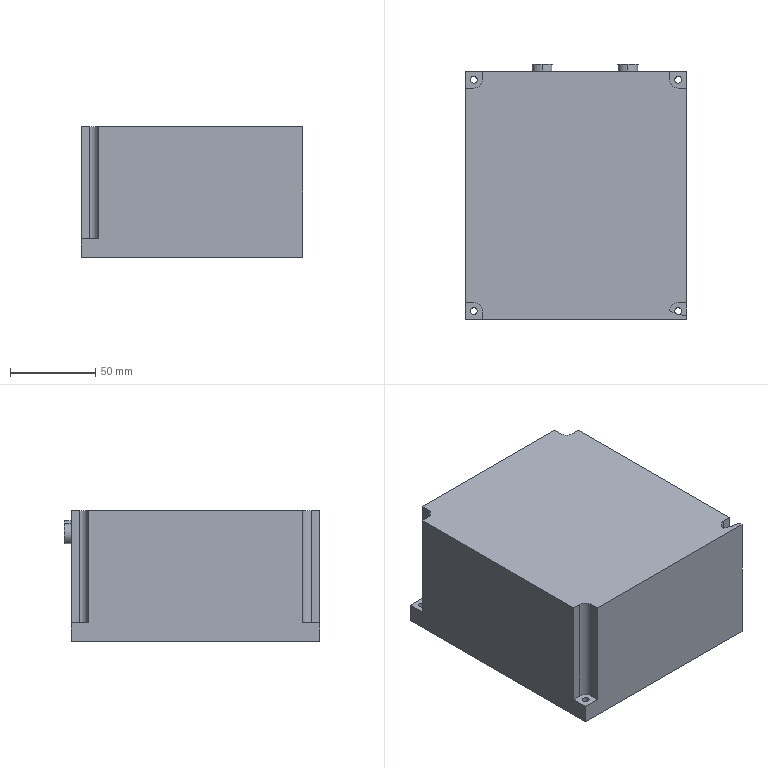Part | SolidWorks | features ICE 2, Extrusion 1 | 1 solid | 37 faces | box 130 x 150 x 77 mm | volume 1439024 mm3 | plane 21 | cylinder 16 | commonest cylinder face diameters 4 x8 10 x4 11.874 x2 11.972 x2
STEP:
#1=CARTESIAN_POINT('',(95.565,150.,59.228));
#2=VERTEX_POINT('',#1);
#3=CARTESIAN_POINT('',(95.565,150.,71.102));
#4=VERTEX_POINT('',#3);
#5=CARTESIAN_POINT('',(95.565,150.,65.165));
#6=DIRECTION('',(0.,-1.,0.));
#7=DIRECTION('',(0.,0.,-1.));
#8=AXIS2_PLACEMENT_3D('',#5,#6,#7);
#9=CIRCLE('',#8,5.937);
#10=EDGE_CURVE('',#2,#4,#9,.T.);
#11=ORIENTED_EDGE('',*,*,#10,.T.);
#12=CARTESIAN_POINT('',(95.565,146.,71.102));
#13=VERTEX_POINT('',#12);
#14=CARTESIAN_POINT('',(95.565,150.,71.102));
#15=DIRECTION('',(0.,-1.,0.));
#16=VECTOR('',#15,1000.);
#17=LINE('',#14,#16);
#18=EDGE_CURVE('',#4,#13,#17,.T.);
#19=ORIENTED_EDGE('',*,*,#18,.T.);
#20=CARTESIAN_POINT('',(95.565,146.,59.228));
#21=VERTEX_POINT('',#20);
#22=CARTESIAN_POINT('',(95.565,146.,65.165));
#23=DIRECTION('',(0.,-1.,0.));
#24=DIRECTION('',(0.,0.,-1.));
#25=AXIS2_PLACEMENT_3D('',#22,#23,#24);
#26=CIRCLE('',#25,5.937);
#27=EDGE_CURVE('',#21,#13,#26,.T.);
#28=ORIENTED_EDGE('',*,*,#27,.F.);
#29=CARTESIAN_POINT('',(95.565,150.,59.228));
#30=DIRECTION('',(0.,-1.,0.));
#31=VECTOR('',#30,1000.);
#32=LINE('',#29,#31);
#33=EDGE_CURVE('',#2,#21,#32,.T.);
#34=ORIENTED_EDGE('',*,*,#33,.F.);
#35=EDGE_LOOP('',(#11,#19,#28,#34));
#36=FACE_OUTER_BOUND('',#35,.T.);
#37=CARTESIAN_POINT('',(95.565,150.,65.165));
#38=DIRECTION('',(0.,-1.,0.));
#39=DIRECTION('',(0.,0.,-1.));
#40=AXIS2_PLACEMENT_3D('',#37,#38,#39);
#41=CYLINDRICAL_SURFACE('',#40,5.937);
#42=ADVANCED_FACE('',(#36),#41,.T.);
#43=CARTESIAN_POINT('',(45.097,150.,57.435));
#44=VERTEX_POINT('',#43);
#45=CARTESIAN_POINT('',(45.097,150.,69.406));
#46=VERTEX_POINT('',#45);
#47=CARTESIAN_POINT('',(45.097,150.,63.42));
#48=DIRECTION('',(0.,-1.,0.));
#49=DIRECTION('',(0.,0.,-1.));
#50=AXIS2_PLACEMENT_3D('',#47,#48,#49);
#51=CIRCLE('',#50,5.986);
#52=EDGE_CURVE('',#44,#46,#51,.T.);
#53=ORIENTED_EDGE('',*,*,#52,.T.);
#54=CARTESIAN_POINT('',(45.097,146.,69.406));
#55=VERTEX_POINT('',#54);
#56=CARTESIAN_POINT('',(45.097,150.,69.406));
#57=DIRECTION('',(0.,-1.,0.));
#58=VECTOR('',#57,1000.);
#59=LINE('',#56,#58);
#60=EDGE_CURVE('',#46,#55,#59,.T.);
#61=ORIENTED_EDGE('',*,*,#60,.T.);
#62=CARTESIAN_POINT('',(45.097,146.,57.435));
#63=VERTEX_POINT('',#62);
#64=CARTESIAN_POINT('',(45.097,146.,63.42));
#65=DIRECTION('',(0.,-1.,0.));
#66=DIRECTION('',(0.,0.,-1.));
#67=AXIS2_PLACEMENT_3D('',#64,#65,#66);
#68=CIRCLE('',#67,5.986);
#69=EDGE_CURVE('',#63,#55,#68,.T.);
#70=ORIENTED_EDGE('',*,*,#69,.F.);
#71=CARTESIAN_POINT('',(45.097,150.,57.435));
#72=DIRECTION('',(0.,-1.,0.));
#73=VECTOR('',#72,1000.);
#74=LINE('',#71,#73);
#75=EDGE_CURVE('',#44,#63,#74,.T.);
#76=ORIENTED_EDGE('',*,*,#75,.F.);
#77=EDGE_LOOP('',(#53,#61,#70,#76));
#78=FACE_OUTER_BOUND('',#77,.T.);
#79=CARTESIAN_POINT('',(45.097,150.,63.42));
#80=DIRECTION('',(0.,-1.,0.));
#81=DIRECTION('',(0.,0.,-1.));
#82=AXIS2_PLACEMENT_3D('',#79,#80,#81);
#83=CYLINDRICAL_SURFACE('',#82,5.986);
#84=ADVANCED_FACE('',(#78),#83,.T.);
#85=CARTESIAN_POINT('',(125.827,3.179,11.));
#86=VERTEX_POINT('',#85);
#87=CARTESIAN_POINT('',(127.,5.,11.));
#88=VERTEX_POINT('',#87);
#89=CARTESIAN_POINT('',(125.,5.,11.));
#90=DIRECTION('',(0.,0.,1.));
#91=DIRECTION('',(1.,0.,0.));
#92=AXIS2_PLACEMENT_3D('',#89,#90,#91);
#93=CIRCLE('',#92,2.);
#94=EDGE_CURVE('',#86,#88,#93,.T.);
#95=ORIENTED_EDGE('',*,*,#94,.T.);
#96=CARTESIAN_POINT('',(127.,5.,0.));
#97=VERTEX_POINT('',#96);
#98=CARTESIAN_POINT('',(127.,5.,77.));
#99=DIRECTION('',(0.,0.,-1.));
#100=VECTOR('',#99,1000.);
#101=LINE('',#98,#100);
#102=EDGE_CURVE('',#88,#97,#101,.T.);
#103=ORIENTED_EDGE('',*,*,#102,.T.);
#104=CARTESIAN_POINT('',(123.,5.,0.));
#105=VERTEX_POINT('',#104);
#106=CARTESIAN_POINT('',(125.,5.,0.));
#107=DIRECTION('',(0.,0.,1.));
#108=DIRECTION('',(1.,0.,0.));
#109=AXIS2_PLACEMENT_3D('',#106,#107,#108);
#110=CIRCLE('',#109,2.);
#111=EDGE_CURVE('',#105,#97,#110,.T.);
#112=ORIENTED_EDGE('',*,*,#111,.F.);
#113=CARTESIAN_POINT('',(123.,5.,11.));
#114=VERTEX_POINT('',#113);
#115=CARTESIAN_POINT('',(123.,5.,77.));
#116=DIRECTION('',(0.,0.,-1.));
#117=VECTOR('',#116,1000.);
#118=LINE('',#115,#117);
#119=EDGE_CURVE('',#114,#105,#118,.T.);
#120=ORIENTED_EDGE('',*,*,#119,.F.);
#121=CARTESIAN_POINT('',(123.283,3.974,11.));
#122=VERTEX_POINT('',#121);
#123=CARTESIAN_POINT('',(125.,5.,11.));
#124=DIRECTION('',(0.,0.,1.));
#125=DIRECTION('',(1.,0.,0.));
#126=AXIS2_PLACEMENT_3D('',#123,#124,#125);
#127=CIRCLE('',#126,2.);
#128=EDGE_CURVE('',#114,#122,#127,.T.);
#129=ORIENTED_EDGE('',*,*,#128,.T.);
#130=CARTESIAN_POINT('',(123.283,3.974,77.));
#131=VERTEX_POINT('',#130);
#132=CARTESIAN_POINT('',(123.283,3.974,77.));
#133=DIRECTION('',(0.,0.,-1.));
#134=VECTOR('',#133,1000.);
#135=LINE('',#132,#134);
#136=EDGE_CURVE('',#131,#122,#135,.T.);
#137=ORIENTED_EDGE('',*,*,#136,.F.);
#138=CARTESIAN_POINT('',(125.827,3.179,77.));
#139=VERTEX_POINT('',#138);
#140=CARTESIAN_POINT('',(125.,5.,77.));
#141=DIRECTION('',(0.,0.,1.));
#142=DIRECTION('',(1.,0.,0.));
#143=AXIS2_PLACEMENT_3D('',#140,#141,#142);
#144=CIRCLE('',#143,2.);
#145=EDGE_CURVE('',#131,#139,#144,.T.);
#146=ORIENTED_EDGE('',*,*,#145,.T.);
#147=CARTESIAN_POINT('',(125.827,3.179,77.));
#148=DIRECTION('',(0.,0.,1.));
#149=VECTOR('',#148,1000.);
#150=LINE('',#147,#149);
#151=EDGE_CURVE('',#86,#139,#150,.T.);
#152=ORIENTED_EDGE('',*,*,#151,.F.);
#153=EDGE_LOOP('',(#95,#103,#112,#120,#129,#137,#146,#152));
#154=FACE_OUTER_BOUND('',#153,.T.);
#155=CARTESIAN_POINT('',(125.,5.,77.));
#156=DIRECTION('',(0.,0.,-1.));
#157=DIRECTION('',(-1.,0.,0.));
#158=AXIS2_PLACEMENT_3D('',#155,#156,#157);
#159=CYLINDRICAL_SURFACE('',#158,2.);
#160=ADVANCED_FACE('',(#154),#159,.F.);
#161=CARTESIAN_POINT('',(123.,141.,11.));
#162=VERTEX_POINT('',#161);
#163=CARTESIAN_POINT('',(127.,141.,11.));
#164=VERTEX_POINT('',#163);
#165=CARTESIAN_POINT('',(125.,141.,11.));
#166=DIRECTION('',(0.,0.,1.));
#167=DIRECTION('',(1.,0.,0.));
#168=AXIS2_PLACEMENT_3D('',#165,#166,#167);
#169=CIRCLE('',#168,2.);
#170=EDGE_CURVE('',#162,#164,#169,.T.);
#171=ORIENTED_EDGE('',*,*,#170,.T.);
#172=CARTESIAN_POINT('',(127.,141.,0.));
#173=VERTEX_POINT('',#172);
#174=CARTESIAN_POINT('',(127.,141.,77.));
#175=DIRECTION('',(0.,0.,-1.));
#176=VECTOR('',#175,1000.);
#177=LINE('',#174,#176);
#178=EDGE_CURVE('',#164,#173,#177,.T.);
#179=ORIENTED_EDGE('',*,*,#178,.T.);
#180=CARTESIAN_POINT('',(123.,141.,0.));
#181=VERTEX_POINT('',#180);
#182=CARTESIAN_POINT('',(125.,141.,0.));
#183=DIRECTION('',(0.,0.,1.));
#184=DIRECTION('',(1.,0.,0.));
#185=AXIS2_PLACEMENT_3D('',#182,#183,#184);
#186=CIRCLE('',#185,2.);
#187=EDGE_CURVE('',#181,#173,#186,.T.);
#188=ORIENTED_EDGE('',*,*,#187,.F.);
#189=CARTESIAN_POINT('',(123.,141.,77.));
#190=DIRECTION('',(0.,0.,-1.));
#191=VECTOR('',#190,1000.);
#192=LINE('',#189,#191);
#193=EDGE_CURVE('',#162,#181,#192,.T.);
#194=ORIENTED_EDGE('',*,*,#193,.F.);
#195=EDGE_LOOP('',(#171,#179,#188,#194));
#196=FACE_OUTER_BOUND('',#195,.T.);
#197=CARTESIAN_POINT('',(125.,141.,77.));
#198=DIRECTION('',(0.,0.,-1.));
#199=DIRECTION('',(-1.,0.,0.));
#200=AXIS2_PLACEMENT_3D('',#197,#198,#199);
#201=CYLINDRICAL_SURFACE('',#200,2.);
#202=ADVANCED_FACE('',(#196),#201,.F.);
#203=CARTESIAN_POINT('',(3.,5.,11.));
#204=VERTEX_POINT('',#203);
#205=CARTESIAN_POINT('',(7.,5.,11.));
#206=VERTEX_POINT('',#205);
#207=CARTESIAN_POINT('',(5.,5.,11.));
#208=DIRECTION('',(0.,0.,1.));
#209=DIRECTION('',(1.,0.,0.));
#210=AXIS2_PLACEMENT_3D('',#207,#208,#209);
#211=CIRCLE('',#210,2.);
#212=EDGE_CURVE('',#204,#206,#211,.T.);
#213=ORIENTED_EDGE('',*,*,#212,.T.);
#214=CARTESIAN_POINT('',(7.,5.,0.));
#215=VERTEX_POINT('',#214);
#216=CARTESIAN_POINT('',(7.,5.,77.));
#217=DIRECTION('',(0.,0.,-1.));
#218=VECTOR('',#217,1000.);
#219=LINE('',#216,#218);
#220=EDGE_CURVE('',#206,#215,#219,.T.);
#221=ORIENTED_EDGE('',*,*,#220,.T.);
#222=CARTESIAN_POINT('',(3.,5.,0.));
#223=VERTEX_POINT('',#222);
#224=CARTESIAN_POINT('',(5.,5.,0.));
#225=DIRECTION('',(0.,0.,1.));
#226=DIRECTION('',(1.,0.,0.));
#227=AXIS2_PLACEMENT_3D('',#224,#225,#226);
#228=CIRCLE('',#227,2.);
#229=EDGE_CURVE('',#223,#215,#228,.T.);
#230=ORIENTED_EDGE('',*,*,#229,.F.);
#231=CARTESIAN_POINT('',(3.,5.,77.));
#232=DIRECTION('',(0.,0.,-1.));
#233=VECTOR('',#232,1000.);
#234=LINE('',#231,#233);
#235=EDGE_CURVE('',#204,#223,#234,.T.);
#236=ORIENTED_EDGE('',*,*,#235,.F.);
#237=EDGE_LOOP('',(#213,#221,#230,#236));
#238=FACE_OUTER_BOUND('',#237,.T.);
#239=CARTESIAN_POINT('',(5.,5.,77.));
#240=DIRECTION('',(0.,0.,-1.));
#241=DIRECTION('',(-1.,0.,0.));
#242=AXIS2_PLACEMENT_3D('',#239,#240,#241);
#243=CYLINDRICAL_SURFACE('',#242,2.);
#244=ADVANCED_FACE('',(#238),#243,.F.);
#245=CARTESIAN_POINT('',(3.,141.,11.));
#246=VERTEX_POINT('',#245);
#247=CARTESIAN_POINT('',(7.,141.,11.));
#248=VERTEX_POINT('',#247);
#249=CARTESIAN_POINT('',(5.,141.,11.));
#250=DIRECTION('',(0.,0.,1.));
#251=DIRECTION('',(1.,0.,0.));
#252=AXIS2_PLACEMENT_3D('',#249,#250,#251);
#253=CIRCLE('',#252,2.);
#254=EDGE_CURVE('',#246,#248,#253,.T.);
#255=ORIENTED_EDGE('',*,*,#254,.T.);
#256=CARTESIAN_POINT('',(7.,141.,0.));
#257=VERTEX_POINT('',#256);
#258=CARTESIAN_POINT('',(7.,141.,77.));
#259=DIRECTION('',(0.,0.,-1.));
#260=VECTOR('',#259,1000.);
#261=LINE('',#258,#260);
#262=EDGE_CURVE('',#248,#257,#261,.T.);
#263=ORIENTED_EDGE('',*,*,#262,.T.);
#264=CARTESIAN_POINT('',(3.,141.,0.));
#265=VERTEX_POINT('',#264);
#266=CARTESIAN_POINT('',(5.,141.,0.));
#267=DIRECTION('',(0.,0.,1.));
#268=DIRECTION('',(1.,0.,0.));
#269=AXIS2_PLACEMENT_3D('',#266,#267,#268);
#270=CIRCLE('',#269,2.);
#271=EDGE_CURVE('',#265,#257,#270,.T.);
#272=ORIENTED_EDGE('',*,*,#271,.F.);
#273=CARTESIAN_POINT('',(3.,141.,77.));
#274=DIRECTION('',(0.,0.,-1.));
#275=VECTOR('',#274,1000.);
#276=LINE('',#273,#275);
#277=EDGE_CURVE('',#246,#265,#276,.T.);
#278=ORIENTED_EDGE('',*,*,#277,.F.);
#279=EDGE_LOOP('',(#255,#263,#272,#278));
#280=FACE_OUTER_BOUND('',#279,.T.);
#281=CARTESIAN_POINT('',(5.,141.,77.));
#282=DIRECTION('',(0.,0.,-1.));
#283=DIRECTION('',(-1.,0.,0.));
#284=AXIS2_PLACEMENT_3D('',#281,#282,#283);
#285=CYLINDRICAL_SURFACE('',#284,2.);
#286=ADVANCED_FACE('',(#280),#285,.F.);
#287=ORIENTED_EDGE('',*,*,#262,.F.);
#288=CARTESIAN_POINT('',(5.,141.,11.));
#289=DIRECTION('',(0.,0.,1.));
#290=DIRECTION('',(1.,0.,0.));
#291=AXIS2_PLACEMENT_3D('',#288,#289,#290);
#292=CIRCLE('',#291,2.);
#293=EDGE_CURVE('',#248,#246,#292,.T.);
#294=ORIENTED_EDGE('',*,*,#293,.T.);
#295=ORIENTED_EDGE('',*,*,#277,.T.);
#296=CARTESIAN_POINT('',(5.,141.,0.));
#297=DIRECTION('',(0.,0.,1.));
#298=DIRECTION('',(1.,0.,0.));
#299=AXIS2_PLACEMENT_3D('',#296,#297,#298);
#300=CIRCLE('',#299,2.);
#301=EDGE_CURVE('',#257,#265,#300,.T.);
#302=ORIENTED_EDGE('',*,*,#301,.F.);
#303=EDGE_LOOP('',(#287,#294,#295,#302));
#304=FACE_OUTER_BOUND('',#303,.T.);
#305=CARTESIAN_POINT('',(5.,141.,77.));
#306=DIRECTION('',(0.,0.,-1.));
#307=DIRECTION('',(-1.,0.,0.));
#308=AXIS2_PLACEMENT_3D('',#305,#306,#307);
#309=CYLINDRICAL_SURFACE('',#308,2.);
#310=ADVANCED_FACE('',(#304),#309,.F.);
#311=ORIENTED_EDGE('',*,*,#220,.F.);
#312=CARTESIAN_POINT('',(5.,5.,11.));
#313=DIRECTION('',(0.,0.,1.));
#314=DIRECTION('',(1.,0.,0.));
#315=AXIS2_PLACEMENT_3D('',#312,#313,#314);
#316=CIRCLE('',#315,2.);
#317=EDGE_CURVE('',#206,#204,#316,.T.);
#318=ORIENTED_EDGE('',*,*,#317,.T.);
#319=ORIENTED_EDGE('',*,*,#235,.T.);
#320=CARTESIAN_POINT('',(5.,5.,0.));
#321=DIRECTION('',(0.,0.,1.));
#322=DIRECTION('',(1.,0.,0.));
#323=AXIS2_PLACEMENT_3D('',#320,#321,#322);
#324=CIRCLE('',#323,2.);
#325=EDGE_CURVE('',#215,#223,#324,.T.);
#326=ORIENTED_EDGE('',*,*,#325,.F.);
#327=EDGE_LOOP('',(#311,#318,#319,#326));
#328=FACE_OUTER_BOUND('',#327,.T.);
#329=CARTESIAN_POINT('',(5.,5.,77.));
#330=DIRECTION('',(0.,0.,-1.));
#331=DIRECTION('',(-1.,0.,0.));
#332=AXIS2_PLACEMENT_3D('',#329,#330,#331);
#333=CYLINDRICAL_SURFACE('',#332,2.);
#334=ADVANCED_FACE('',(#328),#333,.F.);
#335=ORIENTED_EDGE('',*,*,#178,.F.);
#336=CARTESIAN_POINT('',(125.,141.,11.));
#337=DIRECTION('',(0.,0.,1.));
#338=DIRECTION('',(1.,0.,0.));
#339=AXIS2_PLACEMENT_3D('',#336,#337,#338);
#340=CIRCLE('',#339,2.);
#341=EDGE_CURVE('',#164,#162,#340,.T.);
#342=ORIENTED_EDGE('',*,*,#341,.T.);
#343=ORIENTED_EDGE('',*,*,#193,.T.);
#344=CARTESIAN_POINT('',(125.,141.,0.));
#345=DIRECTION('',(0.,0.,1.));
#346=DIRECTION('',(1.,0.,0.));
#347=AXIS2_PLACEMENT_3D('',#344,#345,#346);
#348=CIRCLE('',#347,2.);
#349=EDGE_CURVE('',#173,#181,#348,.T.);
#350=ORIENTED_EDGE('',*,*,#349,.F.);
#351=EDGE_LOOP('',(#335,#342,#343,#350));
#352=FACE_OUTER_BOUND('',#351,.T.);
#353=CARTESIAN_POINT('',(125.,141.,77.));
#354=DIRECTION('',(0.,0.,-1.));
#355=DIRECTION('',(-1.,0.,0.));
#356=AXIS2_PLACEMENT_3D('',#353,#354,#355);
#357=CYLINDRICAL_SURFACE('',#356,2.);
#358=ADVANCED_FACE('',(#352),#357,.F.);
#359=CARTESIAN_POINT('',(5.,136.,77.));
#360=VERTEX_POINT('',#359);
#361=CARTESIAN_POINT('',(10.,141.,77.));
#362=VERTEX_POINT('',#361);
#363=CARTESIAN_POINT('',(5.,141.,77.));
#364=DIRECTION('',(0.,0.,1.));
#365=DIRECTION('',(1.,0.,0.));
#366=AXIS2_PLACEMENT_3D('',#363,#364,#365);
#367=CIRCLE('',#366,5.);
#368=EDGE_CURVE('',#360,#362,#367,.T.);
#369=ORIENTED_EDGE('',*,*,#368,.F.);
#370=CARTESIAN_POINT('',(0.,136.,77.));
#371=VERTEX_POINT('',#370);
#372=CARTESIAN_POINT('',(0.,136.,77.));
#373=DIRECTION('',(1.,0.,0.));
#374=VECTOR('',#373,1000.);
#375=LINE('',#372,#374);
#376=EDGE_CURVE('',#371,#360,#375,.T.);
#377=ORIENTED_EDGE('',*,*,#376,.F.);
#378=CARTESIAN_POINT('',(0.,10.,77.));
#379=VERTEX_POINT('',#378);
#380=CARTESIAN_POINT('',(0.,0.,77.));
#381=DIRECTION('',(0.,-1.,0.));
#382=VECTOR('',#381,1000.);
#383=LINE('',#380,#382);
#384=EDGE_CURVE('',#371,#379,#383,.T.);
#385=ORIENTED_EDGE('',*,*,#384,.T.);
#386=CARTESIAN_POINT('',(5.,10.,77.));
#387=VERTEX_POINT('',#386);
#388=CARTESIAN_POINT('',(0.,10.,77.));
#389=DIRECTION('',(-1.,0.,0.));
#390=VECTOR('',#389,1000.);
#391=LINE('',#388,#390);
#392=EDGE_CURVE('',#387,#379,#391,.T.);
#393=ORIENTED_EDGE('',*,*,#392,.F.);
#394=CARTESIAN_POINT('',(10.,5.,77.));
#395=VERTEX_POINT('',#394);
#396=CARTESIAN_POINT('',(5.,5.,77.));
#397=DIRECTION('',(0.,0.,1.));
#398=DIRECTION('',(1.,0.,0.));
#399=AXIS2_PLACEMENT_3D('',#396,#397,#398);
#400=CIRCLE('',#399,5.);
#401=EDGE_CURVE('',#395,#387,#400,.T.);
#402=ORIENTED_EDGE('',*,*,#401,.F.);
#403=CARTESIAN_POINT('',(10.,0.,77.));
#404=VERTEX_POINT('',#403);
#405=CARTESIAN_POINT('',(10.,5.,77.));
#406=DIRECTION('',(0.,1.,0.));
#407=VECTOR('',#406,1000.);
#408=LINE('',#405,#407);
#409=EDGE_CURVE('',#404,#395,#408,.T.);
#410=ORIENTED_EDGE('',*,*,#409,.F.);
#411=CARTESIAN_POINT('',(130.,0.,77.));
#412=VERTEX_POINT('',#411);
#413=CARTESIAN_POINT('',(0.,0.,77.));
#414=DIRECTION('',(1.,0.,0.));
#415=VECTOR('',#414,1000.);
#416=LINE('',#413,#415);
#417=EDGE_CURVE('',#404,#412,#416,.T.);
#418=ORIENTED_EDGE('',*,*,#417,.T.);
#419=CARTESIAN_POINT('',(130.,1.875,77.));
#420=VERTEX_POINT('',#419);
#421=CARTESIAN_POINT('',(130.,0.,77.));
#422=DIRECTION('',(0.,1.,0.));
#423=VECTOR('',#422,1000.);
#424=LINE('',#421,#423);
#425=EDGE_CURVE('',#412,#420,#424,.T.);
#426=ORIENTED_EDGE('',*,*,#425,.T.);
#427=CARTESIAN_POINT('',(120.,5.,77.));
#428=DIRECTION('',(0.9545,-0.2983,0.));
#429=VECTOR('',#428,1000.);
#430=LINE('',#427,#429);
#431=EDGE_CURVE('',#139,#420,#430,.T.);
#432=ORIENTED_EDGE('',*,*,#431,.F.);
#433=ORIENTED_EDGE('',*,*,#145,.F.);
#434=CARTESIAN_POINT('',(120.,5.,77.));
#435=VERTEX_POINT('',#434);
#436=CARTESIAN_POINT('',(120.,5.,77.));
#437=DIRECTION('',(0.9545,-0.2983,0.));
#438=VECTOR('',#437,1000.);
#439=LINE('',#436,#438);
#440=EDGE_CURVE('',#435,#131,#439,.T.);
#441=ORIENTED_EDGE('',*,*,#440,.F.);
#442=CARTESIAN_POINT('',(125.,10.,77.));
#443=VERTEX_POINT('',#442);
#444=CARTESIAN_POINT('',(125.,5.,77.));
#445=DIRECTION('',(0.,0.,1.));
#446=DIRECTION('',(1.,0.,0.));
#447=AXIS2_PLACEMENT_3D('',#444,#445,#446);
#448=CIRCLE('',#447,5.);
#449=EDGE_CURVE('',#443,#435,#448,.T.);
#450=ORIENTED_EDGE('',*,*,#449,.F.);
#451=CARTESIAN_POINT('',(130.,10.,77.));
#452=VERTEX_POINT('',#451);
#453=CARTESIAN_POINT('',(130.,10.,77.));
#454=DIRECTION('',(-1.,0.,0.));
#455=VECTOR('',#454,1000.);
#456=LINE('',#453,#455);
#457=EDGE_CURVE('',#452,#443,#456,.T.);
#458=ORIENTED_EDGE('',*,*,#457,.F.);
#459=CARTESIAN_POINT('',(130.,136.,77.));
#460=VERTEX_POINT('',#459);
#461=CARTESIAN_POINT('',(130.,0.,77.));
#462=DIRECTION('',(0.,1.,0.));
#463=VECTOR('',#462,1000.);
#464=LINE('',#461,#463);
#465=EDGE_CURVE('',#452,#460,#464,.T.);
#466=ORIENTED_EDGE('',*,*,#465,.T.);
#467=CARTESIAN_POINT('',(125.,136.,77.));
#468=VERTEX_POINT('',#467);
#469=CARTESIAN_POINT('',(130.,136.,77.));
#470=DIRECTION('',(1.,0.,0.));
#471=VECTOR('',#470,1000.);
#472=LINE('',#469,#471);
#473=EDGE_CURVE('',#468,#460,#472,.T.);
#474=ORIENTED_EDGE('',*,*,#473,.F.);
#475=CARTESIAN_POINT('',(120.,141.,77.));
#476=VERTEX_POINT('',#475);
#477=CARTESIAN_POINT('',(125.,141.,77.));
#478=DIRECTION('',(0.,0.,1.));
#479=DIRECTION('',(1.,0.,0.));
#480=AXIS2_PLACEMENT_3D('',#477,#478,#479);
#481=CIRCLE('',#480,5.);
#482=EDGE_CURVE('',#476,#468,#481,.T.);
#483=ORIENTED_EDGE('',*,*,#482,.F.);
#484=CARTESIAN_POINT('',(120.,146.,77.));
#485=VERTEX_POINT('',#484);
#486=CARTESIAN_POINT('',(120.,141.,77.));
#487=DIRECTION('',(0.,-1.,0.));
#488=VECTOR('',#487,1000.);
#489=LINE('',#486,#488);
#490=EDGE_CURVE('',#485,#476,#489,.T.);
#491=ORIENTED_EDGE('',*,*,#490,.F.);
#492=CARTESIAN_POINT('',(10.,146.,77.));
#493=VERTEX_POINT('',#492);
#494=CARTESIAN_POINT('',(0.,146.,77.));
#495=DIRECTION('',(-1.,0.,0.));
#496=VECTOR('',#495,1000.);
#497=LINE('',#494,#496);
#498=EDGE_CURVE('',#485,#493,#497,.T.);
#499=ORIENTED_EDGE('',*,*,#498,.T.);
#500=CARTESIAN_POINT('',(10.,141.,77.));
#501=DIRECTION('',(0.,1.,0.));
#502=VECTOR('',#501,1000.);
#503=LINE('',#500,#502);
#504=EDGE_CURVE('',#362,#493,#503,.T.);
#505=ORIENTED_EDGE('',*,*,#504,.F.);
#506=EDGE_LOOP('',(#369,#377,#385,#393,#402,#410,#418,#426,#432,#433,#441,#450,#458,#466,#474,#483,#491,#499,#505));
#507=FACE_OUTER_BOUND('',#506,.T.);
#508=CARTESIAN_POINT('',(0.,0.,77.));
#509=DIRECTION('',(0.,0.,-1.));
#510=DIRECTION('',(-1.,0.,0.));
#511=AXIS2_PLACEMENT_3D('',#508,#509,#510);
#512=PLANE('',#511);
#513=ADVANCED_FACE('',(#507),#512,.F.);
#514=ORIENTED_EDGE('',*,*,#111,.T.);
#515=CARTESIAN_POINT('',(125.,5.,0.));
#516=DIRECTION('',(0.,0.,1.));
#517=DIRECTION('',(1.,0.,0.));
#518=AXIS2_PLACEMENT_3D('',#515,#516,#517);
#519=CIRCLE('',#518,2.);
#520=EDGE_CURVE('',#97,#105,#519,.T.);
#521=ORIENTED_EDGE('',*,*,#520,.T.);
#522=EDGE_LOOP('',(#514,#521));
#523=FACE_BOUND('',#522,.T.);
#524=ORIENTED_EDGE('',*,*,#271,.T.);
#525=ORIENTED_EDGE('',*,*,#301,.T.);
#526=EDGE_LOOP('',(#524,#525));
#527=FACE_BOUND('',#526,.T.);
#528=CARTESIAN_POINT('',(0.,146.,0.));
#529=VERTEX_POINT('',#528);
#530=CARTESIAN_POINT('',(0.,0.,0.));
#531=VERTEX_POINT('',#530);
#532=CARTESIAN_POINT('',(0.,0.,0.));
#533=DIRECTION('',(0.,-1.,0.));
#534=VECTOR('',#533,1000.);
#535=LINE('',#532,#534);
#536=EDGE_CURVE('',#529,#531,#535,.T.);
#537=ORIENTED_EDGE('',*,*,#536,.F.);
#538=CARTESIAN_POINT('',(130.,146.,0.));
#539=VERTEX_POINT('',#538);
#540=CARTESIAN_POINT('',(0.,146.,0.));
#541=DIRECTION('',(-1.,0.,0.));
#542=VECTOR('',#541,1000.);
#543=LINE('',#540,#542);
#544=EDGE_CURVE('',#539,#529,#543,.T.);
#545=ORIENTED_EDGE('',*,*,#544,.F.);
#546=CARTESIAN_POINT('',(130.,0.,0.));
#547=VERTEX_POINT('',#546);
#548=CARTESIAN_POINT('',(130.,0.,0.));
#549=DIRECTION('',(0.,1.,0.));
#550=VECTOR('',#549,1000.);
#551=LINE('',#548,#550);
#552=EDGE_CURVE('',#547,#539,#551,.T.);
#553=ORIENTED_EDGE('',*,*,#552,.F.);
#554=CARTESIAN_POINT('',(0.,0.,0.));
#555=DIRECTION('',(1.,0.,0.));
#556=VECTOR('',#555,1000.);
#557=LINE('',#554,#556);
#558=EDGE_CURVE('',#531,#547,#557,.T.);
#559=ORIENTED_EDGE('',*,*,#558,.F.);
#560=EDGE_LOOP('',(#537,#545,#553,#559));
#561=FACE_OUTER_BOUND('',#560,.T.);
#562=ORIENTED_EDGE('',*,*,#187,.T.);
#563=ORIENTED_EDGE('',*,*,#349,.T.);
#564=EDGE_LOOP('',(#562,#563));
#565=FACE_BOUND('',#564,.T.);
#566=ORIENTED_EDGE('',*,*,#229,.T.);
#567=ORIENTED_EDGE('',*,*,#325,.T.);
#568=EDGE_LOOP('',(#566,#567));
#569=FACE_BOUND('',#568,.T.);
#570=CARTESIAN_POINT('',(0.,0.,0.));
#571=DIRECTION('',(0.,0.,-1.));
#572=DIRECTION('',(-1.,0.,0.));
#573=AXIS2_PLACEMENT_3D('',#570,#571,#572);
#574=PLANE('',#573);
#575=ADVANCED_FACE('',(#523,#527,#561,#565,#569),#574,.T.);
#576=ORIENTED_EDGE('',*,*,#384,.F.);
#577=CARTESIAN_POINT('',(0.,136.,11.));
#578=VERTEX_POINT('',#577);
#579=CARTESIAN_POINT('',(0.,136.,11.));
#580=DIRECTION('',(0.,0.,1.));
#581=VECTOR('',#580,1000.);
#582=LINE('',#579,#581);
#583=EDGE_CURVE('',#578,#371,#582,.T.);
#584=ORIENTED_EDGE('',*,*,#583,.F.);
#585=CARTESIAN_POINT('',(0.,146.,11.));
#586=VERTEX_POINT('',#585);
#587=CARTESIAN_POINT('',(0.,160.,11.));
#588=DIRECTION('',(0.,-1.,0.));
#589=VECTOR('',#588,1000.);
#590=LINE('',#587,#589);
#591=EDGE_CURVE('',#586,#578,#590,.T.);
#592=ORIENTED_EDGE('',*,*,#591,.F.);
#593=CARTESIAN_POINT('',(0.,146.,77.));
#594=DIRECTION('',(0.,0.,-1.));
#595=VECTOR('',#594,1000.);
#596=LINE('',#593,#595);
#597=EDGE_CURVE('',#586,#529,#596,.T.);
#598=ORIENTED_EDGE('',*,*,#597,.T.);
#599=ORIENTED_EDGE('',*,*,#536,.T.);
#600=CARTESIAN_POINT('',(0.,0.,11.));
#601=VERTEX_POINT('',#600);
#602=CARTESIAN_POINT('',(0.,0.,77.));
#603=DIRECTION('',(0.,0.,-1.));
#604=VECTOR('',#603,1000.);
#605=LINE('',#602,#604);
#606=EDGE_CURVE('',#601,#531,#605,.T.);
#607=ORIENTED_EDGE('',*,*,#606,.F.);
#608=CARTESIAN_POINT('',(0.,10.,11.));
#609=VERTEX_POINT('',#608);
#610=CARTESIAN_POINT('',(0.,0.,11.));
#611=DIRECTION('',(0.,-1.,0.));
#612=VECTOR('',#611,1000.);
#613=LINE('',#610,#612);
#614=EDGE_CURVE('',#609,#601,#613,.T.);
#615=ORIENTED_EDGE('',*,*,#614,.F.);
#616=CARTESIAN_POINT('',(0.,10.,11.));
#617=DIRECTION('',(0.,0.,1.));
#618=VECTOR('',#617,1000.);
#619=LINE('',#616,#618);
#620=EDGE_CURVE('',#609,#379,#619,.T.);
#621=ORIENTED_EDGE('',*,*,#620,.T.);
#622=EDGE_LOOP('',(#576,#584,#592,#598,#599,#607,#615,#621));
#623=FACE_OUTER_BOUND('',#622,.T.);
#624=CARTESIAN_POINT('',(0.,0.,77.));
#625=DIRECTION('',(1.,0.,0.));
#626=DIRECTION('',(0.,0.,-1.));
#627=AXIS2_PLACEMENT_3D('',#624,#625,#626);
#628=PLANE('',#627);
#629=ADVANCED_FACE('',(#623),#628,.F.);
#630=ORIENTED_EDGE('',*,*,#417,.F.);
#631=CARTESIAN_POINT('',(10.,0.,11.));
#632=VERTEX_POINT('',#631);
#633=CARTESIAN_POINT('',(10.,0.,11.));
#634=DIRECTION('',(0.,0.,1.));
#635=VECTOR('',#634,1000.);
#636=LINE('',#633,#635);
#637=EDGE_CURVE('',#632,#404,#636,.T.);
#638=ORIENTED_EDGE('',*,*,#637,.F.);
#639=CARTESIAN_POINT('',(10.,0.,11.));
#640=DIRECTION('',(1.,0.,0.));
#641=VECTOR('',#640,1000.);
#642=LINE('',#639,#641);
#643=EDGE_CURVE('',#601,#632,#642,.T.);
#644=ORIENTED_EDGE('',*,*,#643,.F.);
#645=ORIENTED_EDGE('',*,*,#606,.T.);
#646=ORIENTED_EDGE('',*,*,#558,.T.);
#647=CARTESIAN_POINT('',(130.,0.,77.));
#648=DIRECTION('',(0.,0.,-1.));
#649=VECTOR('',#648,1000.);
#650=LINE('',#647,#649);
#651=EDGE_CURVE('',#412,#547,#650,.T.);
#652=ORIENTED_EDGE('',*,*,#651,.F.);
#653=EDGE_LOOP('',(#630,#638,#644,#645,#646,#652));
#654=FACE_OUTER_BOUND('',#653,.T.);
#655=CARTESIAN_POINT('',(0.,0.,77.));
#656=DIRECTION('',(0.,1.,0.));
#657=DIRECTION('',(0.,0.,1.));
#658=AXIS2_PLACEMENT_3D('',#655,#656,#657);
#659=PLANE('',#658);
#660=ADVANCED_FACE('',(#654),#659,.F.);
#661=ORIENTED_EDGE('',*,*,#465,.F.);
#662=CARTESIAN_POINT('',(130.,10.,11.));
#663=VERTEX_POINT('',#662);
#664=CARTESIAN_POINT('',(130.,10.,11.));
#665=DIRECTION('',(0.,0.,1.));
#666=VECTOR('',#665,1000.);
#667=LINE('',#664,#666);
#668=EDGE_CURVE('',#663,#452,#667,.T.);
#669=ORIENTED_EDGE('',*,*,#668,.F.);
#670=CARTESIAN_POINT('',(130.,1.875,11.));
#671=VERTEX_POINT('',#670);
#672=CARTESIAN_POINT('',(130.,0.,11.));
#673=DIRECTION('',(0.,1.,0.));
#674=VECTOR('',#673,1000.);
#675=LINE('',#672,#674);
#676=EDGE_CURVE('',#671,#663,#675,.T.);
#677=ORIENTED_EDGE('',*,*,#676,.F.);
#678=CARTESIAN_POINT('',(130.,1.875,77.));
#679=DIRECTION('',(0.,0.,1.));
#680=VECTOR('',#679,1000.);
#681=LINE('',#678,#680);
#682=EDGE_CURVE('',#671,#420,#681,.T.);
#683=ORIENTED_EDGE('',*,*,#682,.T.);
#684=ORIENTED_EDGE('',*,*,#425,.F.);
#685=ORIENTED_EDGE('',*,*,#651,.T.);
#686=ORIENTED_EDGE('',*,*,#552,.T.);
#687=CARTESIAN_POINT('',(130.,146.,11.));
#688=VERTEX_POINT('',#687);
#689=CARTESIAN_POINT('',(130.,146.,77.));
#690=DIRECTION('',(0.,0.,-1.));
#691=VECTOR('',#690,1000.);
#692=LINE('',#689,#691);
#693=EDGE_CURVE('',#688,#539,#692,.T.);
#694=ORIENTED_EDGE('',*,*,#693,.F.);
#695=CARTESIAN_POINT('',(130.,136.,11.));
#696=VERTEX_POINT('',#695);
#697=CARTESIAN_POINT('',(130.,0.,11.));
#698=DIRECTION('',(0.,1.,0.));
#699=VECTOR('',#698,1000.);
#700=LINE('',#697,#699);
#701=EDGE_CURVE('',#696,#688,#700,.T.);
#702=ORIENTED_EDGE('',*,*,#701,.F.);
#703=CARTESIAN_POINT('',(130.,136.,11.));
#704=DIRECTION('',(0.,0.,1.));
#705=VECTOR('',#704,1000.);
#706=LINE('',#703,#705);
#707=EDGE_CURVE('',#696,#460,#706,.T.);
#708=ORIENTED_EDGE('',*,*,#707,.T.);
#709=EDGE_LOOP('',(#661,#669,#677,#683,#684,#685,#686,#694,#702,#708));
#710=FACE_OUTER_BOUND('',#709,.T.);
#711=CARTESIAN_POINT('',(130.,0.,77.));
#712=DIRECTION('',(-1.,0.,0.));
#713=DIRECTION('',(0.,0.,1.));
#714=AXIS2_PLACEMENT_3D('',#711,#712,#713);
#715=PLANE('',#714);
#716=ADVANCED_FACE('',(#710),#715,.F.);
#717=ORIENTED_EDGE('',*,*,#27,.T.);
#718=CARTESIAN_POINT('',(95.565,146.,65.165));
#719=DIRECTION('',(0.,-1.,0.));
#720=DIRECTION('',(0.,0.,-1.));
#721=AXIS2_PLACEMENT_3D('',#718,#719,#720);
#722=CIRCLE('',#721,5.937);
#723=EDGE_CURVE('',#13,#21,#722,.T.);
#724=ORIENTED_EDGE('',*,*,#723,.T.);
#725=EDGE_LOOP('',(#717,#724));
#726=FACE_BOUND('',#725,.T.);
#727=ORIENTED_EDGE('',*,*,#69,.T.);
#728=CARTESIAN_POINT('',(45.097,146.,63.42));
#729=DIRECTION('',(0.,-1.,0.));
#730=DIRECTION('',(0.,0.,-1.));
#731=AXIS2_PLACEMENT_3D('',#728,#729,#730);
#732=CIRCLE('',#731,5.986);
#733=EDGE_CURVE('',#55,#63,#732,.T.);
#734=ORIENTED_EDGE('',*,*,#733,.T.);
#735=EDGE_LOOP('',(#727,#734));
#736=FACE_BOUND('',#735,.T.);
#737=CARTESIAN_POINT('',(10.,146.,11.));
#738=VERTEX_POINT('',#737);
#739=CARTESIAN_POINT('',(0.,146.,11.));
#740=DIRECTION('',(-1.,0.,0.));
#741=VECTOR('',#740,1000.);
#742=LINE('',#739,#741);
#743=EDGE_CURVE('',#738,#586,#742,.T.);
#744=ORIENTED_EDGE('',*,*,#743,.F.);
#745=CARTESIAN_POINT('',(10.,146.,11.));
#746=DIRECTION('',(0.,0.,1.));
#747=VECTOR('',#746,1000.);
#748=LINE('',#745,#747);
#749=EDGE_CURVE('',#738,#493,#748,.T.);
#750=ORIENTED_EDGE('',*,*,#749,.T.);
#751=ORIENTED_EDGE('',*,*,#498,.F.);
#752=CARTESIAN_POINT('',(120.,146.,11.));
#753=VERTEX_POINT('',#752);
#754=CARTESIAN_POINT('',(120.,146.,11.));
#755=DIRECTION('',(0.,0.,1.));
#756=VECTOR('',#755,1000.);
#757=LINE('',#754,#756);
#758=EDGE_CURVE('',#753,#485,#757,.T.);
#759=ORIENTED_EDGE('',*,*,#758,.F.);
#760=CARTESIAN_POINT('',(0.,146.,11.));
#761=DIRECTION('',(-1.,0.,0.));
#762=VECTOR('',#761,1000.);
#763=LINE('',#760,#762);
#764=EDGE_CURVE('',#688,#753,#763,.T.);
#765=ORIENTED_EDGE('',*,*,#764,.F.);
#766=ORIENTED_EDGE('',*,*,#693,.T.);
#767=ORIENTED_EDGE('',*,*,#544,.T.);
#768=ORIENTED_EDGE('',*,*,#597,.F.);
#769=EDGE_LOOP('',(#744,#750,#751,#759,#765,#766,#767,#768));
#770=FACE_OUTER_BOUND('',#769,.T.);
#771=CARTESIAN_POINT('',(0.,146.,77.));
#772=DIRECTION('',(0.,-1.,0.));
#773=DIRECTION('',(0.,0.,-1.));
#774=AXIS2_PLACEMENT_3D('',#771,#772,#773);
#775=PLANE('',#774);
#776=ADVANCED_FACE('',(#726,#736,#770),#775,.F.);
#777=ORIENTED_EDGE('',*,*,#102,.F.);
#778=CARTESIAN_POINT('',(125.,5.,11.));
#779=DIRECTION('',(0.,0.,1.));
#780=DIRECTION('',(1.,0.,0.));
#781=AXIS2_PLACEMENT_3D('',#778,#779,#780);
#782=CIRCLE('',#781,2.);
#783=EDGE_CURVE('',#88,#114,#782,.T.);
#784=ORIENTED_EDGE('',*,*,#783,.T.);
#785=ORIENTED_EDGE('',*,*,#119,.T.);
#786=ORIENTED_EDGE('',*,*,#520,.F.);
#787=EDGE_LOOP('',(#777,#784,#785,#786));
#788=FACE_OUTER_BOUND('',#787,.T.);
#789=CARTESIAN_POINT('',(125.,5.,77.));
#790=DIRECTION('',(0.,0.,-1.));
#791=DIRECTION('',(-1.,0.,0.));
#792=AXIS2_PLACEMENT_3D('',#789,#790,#791);
#793=CYLINDRICAL_SURFACE('',#792,2.);
#794=ADVANCED_FACE('',(#788),#793,.F.);
#795=ORIENTED_EDGE('',*,*,#170,.F.);
#796=ORIENTED_EDGE('',*,*,#341,.F.);
#797=EDGE_LOOP('',(#795,#796));
#798=FACE_BOUND('',#797,.T.);
#799=ORIENTED_EDGE('',*,*,#701,.T.);
#800=ORIENTED_EDGE('',*,*,#764,.T.);
#801=CARTESIAN_POINT('',(120.,141.,11.));
#802=VERTEX_POINT('',#801);
#803=CARTESIAN_POINT('',(120.,141.,11.));
#804=DIRECTION('',(0.,-1.,0.));
#805=VECTOR('',#804,1000.);
#806=LINE('',#803,#805);
#807=EDGE_CURVE('',#753,#802,#806,.T.);
#808=ORIENTED_EDGE('',*,*,#807,.T.);
#809=CARTESIAN_POINT('',(125.,136.,11.));
#810=VERTEX_POINT('',#809);
#811=CARTESIAN_POINT('',(125.,141.,11.));
#812=DIRECTION('',(0.,0.,1.));
#813=DIRECTION('',(1.,0.,0.));
#814=AXIS2_PLACEMENT_3D('',#811,#812,#813);
#815=CIRCLE('',#814,5.);
#816=EDGE_CURVE('',#802,#810,#815,.T.);
#817=ORIENTED_EDGE('',*,*,#816,.T.);
#818=CARTESIAN_POINT('',(130.,136.,11.));
#819=DIRECTION('',(1.,0.,0.));
#820=VECTOR('',#819,1000.);
#821=LINE('',#818,#820);
#822=EDGE_CURVE('',#810,#696,#821,.T.);
#823=ORIENTED_EDGE('',*,*,#822,.T.);
#824=EDGE_LOOP('',(#799,#800,#808,#817,#823));
#825=FACE_OUTER_BOUND('',#824,.T.);
#826=CARTESIAN_POINT('',(125.,141.,11.));
#827=DIRECTION('',(0.,0.,1.));
#828=DIRECTION('',(1.,0.,0.));
#829=AXIS2_PLACEMENT_3D('',#826,#827,#828);
#830=PLANE('',#829);
#831=ADVANCED_FACE('',(#798,#825),#830,.T.);
#832=ORIENTED_EDGE('',*,*,#482,.T.);
#833=CARTESIAN_POINT('',(125.,136.,11.));
#834=DIRECTION('',(0.,0.,1.));
#835=VECTOR('',#834,1000.);
#836=LINE('',#833,#835);
#837=EDGE_CURVE('',#810,#468,#836,.T.);
#838=ORIENTED_EDGE('',*,*,#837,.F.);
#839=ORIENTED_EDGE('',*,*,#816,.F.);
#840=CARTESIAN_POINT('',(120.,141.,11.));
#841=DIRECTION('',(0.,0.,1.));
#842=VECTOR('',#841,1000.);
#843=LINE('',#840,#842);
#844=EDGE_CURVE('',#802,#476,#843,.T.);
#845=ORIENTED_EDGE('',*,*,#844,.T.);
#846=EDGE_LOOP('',(#832,#838,#839,#845));
#847=FACE_OUTER_BOUND('',#846,.T.);
#848=CARTESIAN_POINT('',(125.,141.,11.));
#849=DIRECTION('',(0.,0.,1.));
#850=DIRECTION('',(1.,0.,0.));
#851=AXIS2_PLACEMENT_3D('',#848,#849,#850);
#852=CYLINDRICAL_SURFACE('',#851,5.);
#853=ADVANCED_FACE('',(#847),#852,.F.);
#854=ORIENTED_EDGE('',*,*,#490,.T.);
#855=ORIENTED_EDGE('',*,*,#844,.F.);
#856=ORIENTED_EDGE('',*,*,#807,.F.);
#857=ORIENTED_EDGE('',*,*,#758,.T.);
#858=EDGE_LOOP('',(#854,#855,#856,#857));
#859=FACE_OUTER_BOUND('',#858,.T.);
#860=CARTESIAN_POINT('',(120.,141.,11.));
#861=DIRECTION('',(-1.,0.,0.));
#862=DIRECTION('',(0.,-1.,0.));
#863=AXIS2_PLACEMENT_3D('',#860,#861,#862);
#864=PLANE('',#863);
#865=ADVANCED_FACE('',(#859),#864,.F.);
#866=ORIENTED_EDGE('',*,*,#473,.T.);
#867=ORIENTED_EDGE('',*,*,#707,.F.);
#868=ORIENTED_EDGE('',*,*,#822,.F.);
#869=ORIENTED_EDGE('',*,*,#837,.T.);
#870=EDGE_LOOP('',(#866,#867,#868,#869));
#871=FACE_OUTER_BOUND('',#870,.T.);
#872=CARTESIAN_POINT('',(130.,136.,11.));
#873=DIRECTION('',(0.,-1.,0.));
#874=DIRECTION('',(1.,0.,0.));
#875=AXIS2_PLACEMENT_3D('',#872,#873,#874);
#876=PLANE('',#875);
#877=ADVANCED_FACE('',(#871),#876,.F.);
#878=ORIENTED_EDGE('',*,*,#401,.T.);
#879=CARTESIAN_POINT('',(5.,10.,11.));
#880=VERTEX_POINT('',#879);
#881=CARTESIAN_POINT('',(5.,10.,11.));
#882=DIRECTION('',(0.,0.,1.));
#883=VECTOR('',#882,1000.);
#884=LINE('',#881,#883);
#885=EDGE_CURVE('',#880,#387,#884,.T.);
#886=ORIENTED_EDGE('',*,*,#885,.F.);
#887=CARTESIAN_POINT('',(10.,5.,11.));
#888=VERTEX_POINT('',#887);
#889=CARTESIAN_POINT('',(5.,5.,11.));
#890=DIRECTION('',(0.,0.,1.));
#891=DIRECTION('',(1.,0.,0.));
#892=AXIS2_PLACEMENT_3D('',#889,#890,#891);
#893=CIRCLE('',#892,5.);
#894=EDGE_CURVE('',#888,#880,#893,.T.);
#895=ORIENTED_EDGE('',*,*,#894,.F.);
#896=CARTESIAN_POINT('',(10.,5.,11.));
#897=DIRECTION('',(0.,0.,1.));
#898=VECTOR('',#897,1000.);
#899=LINE('',#896,#898);
#900=EDGE_CURVE('',#888,#395,#899,.T.);
#901=ORIENTED_EDGE('',*,*,#900,.T.);
#902=EDGE_LOOP('',(#878,#886,#895,#901));
#903=FACE_OUTER_BOUND('',#902,.T.);
#904=CARTESIAN_POINT('',(5.,5.,11.));
#905=DIRECTION('',(0.,0.,1.));
#906=DIRECTION('',(1.,0.,0.));
#907=AXIS2_PLACEMENT_3D('',#904,#905,#906);
#908=CYLINDRICAL_SURFACE('',#907,5.);
#909=ADVANCED_FACE('',(#903),#908,.F.);
#910=ORIENTED_EDGE('',*,*,#409,.T.);
#911=ORIENTED_EDGE('',*,*,#900,.F.);
#912=CARTESIAN_POINT('',(10.,5.,11.));
#913=DIRECTION('',(0.,1.,0.));
#914=VECTOR('',#913,1000.);
#915=LINE('',#912,#914);
#916=EDGE_CURVE('',#632,#888,#915,.T.);
#917=ORIENTED_EDGE('',*,*,#916,.F.);
#918=ORIENTED_EDGE('',*,*,#637,.T.);
#919=EDGE_LOOP('',(#910,#911,#917,#918));
#920=FACE_OUTER_BOUND('',#919,.T.);
#921=CARTESIAN_POINT('',(10.,5.,11.));
#922=DIRECTION('',(1.,0.,0.));
#923=DIRECTION('',(0.,1.,0.));
#924=AXIS2_PLACEMENT_3D('',#921,#922,#923);
#925=PLANE('',#924);
#926=ADVANCED_FACE('',(#920),#925,.F.);
#927=ORIENTED_EDGE('',*,*,#392,.T.);
#928=ORIENTED_EDGE('',*,*,#620,.F.);
#929=CARTESIAN_POINT('',(0.,10.,11.));
#930=DIRECTION('',(-1.,0.,0.));
#931=VECTOR('',#930,1000.);
#932=LINE('',#929,#931);
#933=EDGE_CURVE('',#880,#609,#932,.T.);
#934=ORIENTED_EDGE('',*,*,#933,.F.);
#935=ORIENTED_EDGE('',*,*,#885,.T.);
#936=EDGE_LOOP('',(#927,#928,#934,#935));
#937=FACE_OUTER_BOUND('',#936,.T.);
#938=CARTESIAN_POINT('',(0.,10.,11.));
#939=DIRECTION('',(0.,1.,0.));
#940=DIRECTION('',(-1.,0.,0.));
#941=AXIS2_PLACEMENT_3D('',#938,#939,#940);
#942=PLANE('',#941);
#943=ADVANCED_FACE('',(#937),#942,.F.);
#944=ORIENTED_EDGE('',*,*,#212,.F.);
#945=ORIENTED_EDGE('',*,*,#317,.F.);
#946=EDGE_LOOP('',(#944,#945));
#947=FACE_BOUND('',#946,.T.);
#948=ORIENTED_EDGE('',*,*,#894,.T.);
#949=ORIENTED_EDGE('',*,*,#933,.T.);
#950=ORIENTED_EDGE('',*,*,#614,.T.);
#951=ORIENTED_EDGE('',*,*,#643,.T.);
#952=ORIENTED_EDGE('',*,*,#916,.T.);
#953=EDGE_LOOP('',(#948,#949,#950,#951,#952));
#954=FACE_OUTER_BOUND('',#953,.T.);
#955=CARTESIAN_POINT('',(5.,5.,11.));
#956=DIRECTION('',(0.,0.,1.));
#957=DIRECTION('',(1.,0.,0.));
#958=AXIS2_PLACEMENT_3D('',#955,#956,#957);
#959=PLANE('',#958);
#960=ADVANCED_FACE('',(#947,#954),#959,.T.);
#961=CARTESIAN_POINT('',(120.,5.,11.));
#962=DIRECTION('',(0.9545,-0.2983,0.));
#963=VECTOR('',#962,1000.);
#964=LINE('',#961,#963);
#965=EDGE_CURVE('',#86,#671,#964,.T.);
#966=ORIENTED_EDGE('',*,*,#965,.F.);
#967=ORIENTED_EDGE('',*,*,#151,.T.);
#968=ORIENTED_EDGE('',*,*,#431,.T.);
#969=ORIENTED_EDGE('',*,*,#682,.F.);
#970=EDGE_LOOP('',(#966,#967,#968,#969));
#971=FACE_OUTER_BOUND('',#970,.T.);
#972=CARTESIAN_POINT('',(120.,5.,11.));
#973=DIRECTION('',(-0.2983,-0.9545,0.));
#974=DIRECTION('',(0.9545,-0.2983,0.));
#975=AXIS2_PLACEMENT_3D('',#972,#973,#974);
#976=PLANE('',#975);
#977=ADVANCED_FACE('',(#971),#976,.F.);
#978=ORIENTED_EDGE('',*,*,#136,.T.);
#979=CARTESIAN_POINT('',(120.,5.,11.));
#980=VERTEX_POINT('',#979);
#981=CARTESIAN_POINT('',(120.,5.,11.));
#982=DIRECTION('',(0.9545,-0.2983,0.));
#983=VECTOR('',#982,1000.);
#984=LINE('',#981,#983);
#985=EDGE_CURVE('',#980,#122,#984,.T.);
#986=ORIENTED_EDGE('',*,*,#985,.F.);
#987=CARTESIAN_POINT('',(120.,5.,11.));
#988=DIRECTION('',(0.,0.,1.));
#989=VECTOR('',#988,1000.);
#990=LINE('',#987,#989);
#991=EDGE_CURVE('',#980,#435,#990,.T.);
#992=ORIENTED_EDGE('',*,*,#991,.T.);
#993=ORIENTED_EDGE('',*,*,#440,.T.);
#994=EDGE_LOOP('',(#978,#986,#992,#993));
#995=FACE_OUTER_BOUND('',#994,.T.);
#996=CARTESIAN_POINT('',(120.,5.,11.));
#997=DIRECTION('',(-0.2983,-0.9545,0.));
#998=DIRECTION('',(0.9545,-0.2983,0.));
#999=AXIS2_PLACEMENT_3D('',#996,#997,#998);
#1000=PLANE('',#999);
#1001=ADVANCED_FACE('',(#995),#1000,.F.);
#1002=ORIENTED_EDGE('',*,*,#676,.T.);
#1003=CARTESIAN_POINT('',(125.,10.,11.));
#1004=VERTEX_POINT('',#1003);
#1005=CARTESIAN_POINT('',(130.,10.,11.));
#1006=DIRECTION('',(-1.,0.,0.));
#1007=VECTOR('',#1006,1000.);
#1008=LINE('',#1005,#1007);
#1009=EDGE_CURVE('',#663,#1004,#1008,.T.);
#1010=ORIENTED_EDGE('',*,*,#1009,.T.);
#1011=CARTESIAN_POINT('',(125.,5.,11.));
#1012=DIRECTION('',(0.,0.,1.));
#1013=DIRECTION('',(1.,0.,0.));
#1014=AXIS2_PLACEMENT_3D('',#1011,#1012,#1013);
#1015=CIRCLE('',#1014,5.);
#1016=EDGE_CURVE('',#1004,#980,#1015,.T.);
#1017=ORIENTED_EDGE('',*,*,#1016,.T.);
#1018=ORIENTED_EDGE('',*,*,#985,.T.);
#1019=ORIENTED_EDGE('',*,*,#128,.F.);
#1020=ORIENTED_EDGE('',*,*,#783,.F.);
#1021=ORIENTED_EDGE('',*,*,#94,.F.);
#1022=ORIENTED_EDGE('',*,*,#965,.T.);
#1023=EDGE_LOOP('',(#1002,#1010,#1017,#1018,#1019,#1020,#1021,#1022));
#1024=FACE_OUTER_BOUND('',#1023,.T.);
#1025=CARTESIAN_POINT('',(125.,5.,11.));
#1026=DIRECTION('',(0.,0.,1.));
#1027=DIRECTION('',(1.,0.,0.));
#1028=AXIS2_PLACEMENT_3D('',#1025,#1026,#1027);
#1029=PLANE('',#1028);
#1030=ADVANCED_FACE('',(#1024),#1029,.T.);
#1031=ORIENTED_EDGE('',*,*,#449,.T.);
#1032=ORIENTED_EDGE('',*,*,#991,.F.);
#1033=ORIENTED_EDGE('',*,*,#1016,.F.);
#1034=CARTESIAN_POINT('',(125.,10.,11.));
#1035=DIRECTION('',(0.,0.,1.));
#1036=VECTOR('',#1035,1000.);
#1037=LINE('',#1034,#1036);
#1038=EDGE_CURVE('',#1004,#443,#1037,.T.);
#1039=ORIENTED_EDGE('',*,*,#1038,.T.);
#1040=EDGE_LOOP('',(#1031,#1032,#1033,#1039));
#1041=FACE_OUTER_BOUND('',#1040,.T.);
#1042=CARTESIAN_POINT('',(125.,5.,11.));
#1043=DIRECTION('',(0.,0.,1.));
#1044=DIRECTION('',(1.,0.,0.));
#1045=AXIS2_PLACEMENT_3D('',#1042,#1043,#1044);
#1046=CYLINDRICAL_SURFACE('',#1045,5.);
#1047=ADVANCED_FACE('',(#1041),#1046,.F.);
#1048=ORIENTED_EDGE('',*,*,#457,.T.);
#1049=ORIENTED_EDGE('',*,*,#1038,.F.);
#1050=ORIENTED_EDGE('',*,*,#1009,.F.);
#1051=ORIENTED_EDGE('',*,*,#668,.T.);
#1052=EDGE_LOOP('',(#1048,#1049,#1050,#1051));
#1053=FACE_OUTER_BOUND('',#1052,.T.);
#1054=CARTESIAN_POINT('',(130.,10.,11.));
#1055=DIRECTION('',(0.,1.,0.));
#1056=DIRECTION('',(-1.,0.,0.));
#1057=AXIS2_PLACEMENT_3D('',#1054,#1055,#1056);
#1058=PLANE('',#1057);
#1059=ADVANCED_FACE('',(#1053),#1058,.F.);
#1060=ORIENTED_EDGE('',*,*,#254,.F.);
#1061=ORIENTED_EDGE('',*,*,#293,.F.);
#1062=EDGE_LOOP('',(#1060,#1061));
#1063=FACE_BOUND('',#1062,.T.);
#1064=ORIENTED_EDGE('',*,*,#743,.T.);
#1065=ORIENTED_EDGE('',*,*,#591,.T.);
#1066=CARTESIAN_POINT('',(5.,136.,11.));
#1067=VERTEX_POINT('',#1066);
#1068=CARTESIAN_POINT('',(0.,136.,11.));
#1069=DIRECTION('',(1.,0.,0.));
#1070=VECTOR('',#1069,1000.);
#1071=LINE('',#1068,#1070);
#1072=EDGE_CURVE('',#578,#1067,#1071,.T.);
#1073=ORIENTED_EDGE('',*,*,#1072,.T.);
#1074=CARTESIAN_POINT('',(10.,141.,11.));
#1075=VERTEX_POINT('',#1074);
#1076=CARTESIAN_POINT('',(5.,141.,11.));
#1077=DIRECTION('',(0.,0.,1.));
#1078=DIRECTION('',(1.,0.,0.));
#1079=AXIS2_PLACEMENT_3D('',#1076,#1077,#1078);
#1080=CIRCLE('',#1079,5.);
#1081=EDGE_CURVE('',#1067,#1075,#1080,.T.);
#1082=ORIENTED_EDGE('',*,*,#1081,.T.);
#1083=CARTESIAN_POINT('',(10.,141.,11.));
#1084=DIRECTION('',(0.,1.,0.));
#1085=VECTOR('',#1084,1000.);
#1086=LINE('',#1083,#1085);
#1087=EDGE_CURVE('',#1075,#738,#1086,.T.);
#1088=ORIENTED_EDGE('',*,*,#1087,.T.);
#1089=EDGE_LOOP('',(#1064,#1065,#1073,#1082,#1088));
#1090=FACE_OUTER_BOUND('',#1089,.T.);
#1091=CARTESIAN_POINT('',(5.,141.,11.));
#1092=DIRECTION('',(0.,0.,1.));
#1093=DIRECTION('',(1.,0.,0.));
#1094=AXIS2_PLACEMENT_3D('',#1091,#1092,#1093);
#1095=PLANE('',#1094);
#1096=ADVANCED_FACE('',(#1063,#1090),#1095,.T.);
#1097=ORIENTED_EDGE('',*,*,#368,.T.);
#1098=CARTESIAN_POINT('',(10.,141.,11.));
#1099=DIRECTION('',(0.,0.,1.));
#1100=VECTOR('',#1099,1000.);
#1101=LINE('',#1098,#1100);
#1102=EDGE_CURVE('',#1075,#362,#1101,.T.);
#1103=ORIENTED_EDGE('',*,*,#1102,.F.);
#1104=ORIENTED_EDGE('',*,*,#1081,.F.);
#1105=CARTESIAN_POINT('',(5.,136.,11.));
#1106=DIRECTION('',(0.,0.,1.));
#1107=VECTOR('',#1106,1000.);
#1108=LINE('',#1105,#1107);
#1109=EDGE_CURVE('',#1067,#360,#1108,.T.);
#1110=ORIENTED_EDGE('',*,*,#1109,.T.);
#1111=EDGE_LOOP('',(#1097,#1103,#1104,#1110));
#1112=FACE_OUTER_BOUND('',#1111,.T.);
#1113=CARTESIAN_POINT('',(5.,141.,11.));
#1114=DIRECTION('',(0.,0.,1.));
#1115=DIRECTION('',(1.,0.,0.));
#1116=AXIS2_PLACEMENT_3D('',#1113,#1114,#1115);
#1117=CYLINDRICAL_SURFACE('',#1116,5.);
#1118=ADVANCED_FACE('',(#1112),#1117,.F.);
#1119=ORIENTED_EDGE('',*,*,#376,.T.);
#1120=ORIENTED_EDGE('',*,*,#1109,.F.);
#1121=ORIENTED_EDGE('',*,*,#1072,.F.);
#1122=ORIENTED_EDGE('',*,*,#583,.T.);
#1123=EDGE_LOOP('',(#1119,#1120,#1121,#1122));
#1124=FACE_OUTER_BOUND('',#1123,.T.);
#1125=CARTESIAN_POINT('',(0.,136.,11.));
#1126=DIRECTION('',(0.,-1.,0.));
#1127=DIRECTION('',(0.,0.,-1.));
#1128=AXIS2_PLACEMENT_3D('',#1125,#1126,#1127);
#1129=PLANE('',#1128);
#1130=ADVANCED_FACE('',(#1124),#1129,.F.);
#1131=ORIENTED_EDGE('',*,*,#504,.T.);
#1132=ORIENTED_EDGE('',*,*,#749,.F.);
#1133=ORIENTED_EDGE('',*,*,#1087,.F.);
#1134=ORIENTED_EDGE('',*,*,#1102,.T.);
#1135=EDGE_LOOP('',(#1131,#1132,#1133,#1134));
#1136=FACE_OUTER_BOUND('',#1135,.T.);
#1137=CARTESIAN_POINT('',(10.,141.,11.));
#1138=DIRECTION('',(1.,0.,0.));
#1139=DIRECTION('',(0.,1.,0.));
#1140=AXIS2_PLACEMENT_3D('',#1137,#1138,#1139);
#1141=PLANE('',#1140);
#1142=ADVANCED_FACE('',(#1136),#1141,.F.);
#1143=ORIENTED_EDGE('',*,*,#60,.F.);
#1144=CARTESIAN_POINT('',(45.097,150.,63.42));
#1145=DIRECTION('',(0.,-1.,0.));
#1146=DIRECTION('',(0.,0.,-1.));
#1147=AXIS2_PLACEMENT_3D('',#1144,#1145,#1146);
#1148=CIRCLE('',#1147,5.986);
#1149=EDGE_CURVE('',#46,#44,#1148,.T.);
#1150=ORIENTED_EDGE('',*,*,#1149,.T.);
#1151=ORIENTED_EDGE('',*,*,#75,.T.);
#1152=ORIENTED_EDGE('',*,*,#733,.F.);
#1153=EDGE_LOOP('',(#1143,#1150,#1151,#1152));
#1154=FACE_OUTER_BOUND('',#1153,.T.);
#1155=CARTESIAN_POINT('',(45.097,150.,63.42));
#1156=DIRECTION('',(0.,-1.,0.));
#1157=DIRECTION('',(0.,0.,-1.));
#1158=AXIS2_PLACEMENT_3D('',#1155,#1156,#1157);
#1159=CYLINDRICAL_SURFACE('',#1158,5.986);
#1160=ADVANCED_FACE('',(#1154),#1159,.T.);
#1161=ORIENTED_EDGE('',*,*,#52,.F.);
#1162=ORIENTED_EDGE('',*,*,#1149,.F.);
#1163=EDGE_LOOP('',(#1161,#1162));
#1164=FACE_OUTER_BOUND('',#1163,.T.);
#1165=CARTESIAN_POINT('',(45.097,150.,63.42));
#1166=DIRECTION('',(0.,-1.,0.));
#1167=DIRECTION('',(0.,0.,-1.));
#1168=AXIS2_PLACEMENT_3D('',#1165,#1166,#1167);
#1169=PLANE('',#1168);
#1170=ADVANCED_FACE('',(#1164),#1169,.F.);
#1171=ORIENTED_EDGE('',*,*,#18,.F.);
#1172=CARTESIAN_POINT('',(95.565,150.,65.165));
#1173=DIRECTION('',(0.,-1.,0.));
#1174=DIRECTION('',(0.,0.,-1.));
#1175=AXIS2_PLACEMENT_3D('',#1172,#1173,#1174);
#1176=CIRCLE('',#1175,5.937);
#1177=EDGE_CURVE('',#4,#2,#1176,.T.);
#1178=ORIENTED_EDGE('',*,*,#1177,.T.);
#1179=ORIENTED_EDGE('',*,*,#33,.T.);
#1180=ORIENTED_EDGE('',*,*,#723,.F.);
#1181=EDGE_LOOP('',(#1171,#1178,#1179,#1180));
#1182=FACE_OUTER_BOUND('',#1181,.T.);
#1183=CARTESIAN_POINT('',(95.565,150.,65.165));
#1184=DIRECTION('',(0.,-1.,0.));
#1185=DIRECTION('',(0.,0.,-1.));
#1186=AXIS2_PLACEMENT_3D('',#1183,#1184,#1185);
#1187=CYLINDRICAL_SURFACE('',#1186,5.937);
#1188=ADVANCED_FACE('',(#1182),#1187,.T.);
#1189=ORIENTED_EDGE('',*,*,#10,.F.);
#1190=ORIENTED_EDGE('',*,*,#1177,.F.);
#1191=EDGE_LOOP('',(#1189,#1190));
#1192=FACE_OUTER_BOUND('',#1191,.T.);
#1193=CARTESIAN_POINT('',(95.565,150.,65.165));
#1194=DIRECTION('',(0.,-1.,0.));
#1195=DIRECTION('',(0.,0.,-1.));
#1196=AXIS2_PLACEMENT_3D('',#1193,#1194,#1195);
#1197=PLANE('',#1196);
#1198=ADVANCED_FACE('',(#1192),#1197,.F.);
#1199=CLOSED_SHELL('',(#42,#84,#160,#202,#244,#286,#310,#334,#358,#513,#575,#629,#660,#716,#776,#794,#831,#853,#865,#877,#909,#926,#943,#960,#977,#1001,#1030,#1047,#1059,#1096,#1118,#1130,#1142,#1160,#1170,#1188,#1198));
#1200=MANIFOLD_SOLID_BREP('',#1199);
#1201=CARTESIAN_POINT('',(0.,0.,0.));
#1202=DIRECTION('',(0.,0.,1.));
#1203=DIRECTION('',(1.,0.,0.));
#1204=AXIS2_PLACEMENT_3D('',#1201,#1202,#1203);
#1205=(LENGTH_UNIT()NAMED_UNIT(*)SI_UNIT(.MILLI.,.METRE.));
#1206=UNCERTAINTY_MEASURE_WITH_UNIT(LENGTH_MEASURE(0.00001),#1205,'','');
#1207=(NAMED_UNIT(*)PLANE_ANGLE_UNIT()SI_UNIT($,.RADIAN.));
#1208=(NAMED_UNIT(*)SI_UNIT($,.STERADIAN.)SOLID_ANGLE_UNIT());
#1209=(GEOMETRIC_REPRESENTATION_CONTEXT(3)GLOBAL_UNCERTAINTY_ASSIGNED_CONTEXT((#1206))GLOBAL_UNIT_ASSIGNED_CONTEXT((#1205,#1207,#1208))REPRESENTATION_CONTEXT('',''));
#1210=ADVANCED_BREP_SHAPE_REPRESENTATION('',(#1200,#1204),#1209);